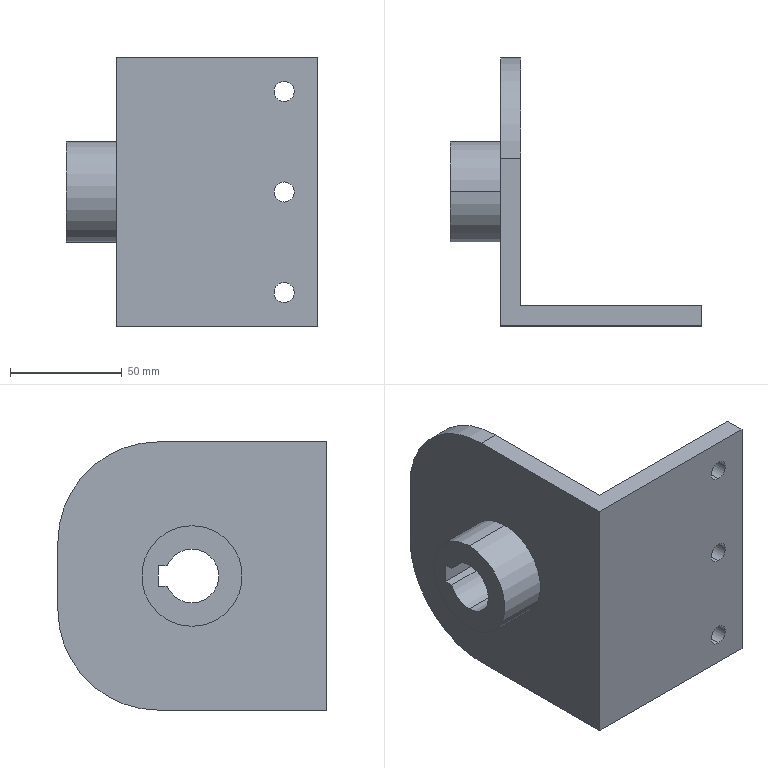Part | SolidWorks | features ICE 2, BaseBody 1 | 1 solid | 25 faces | box 112.5 x 120 x 120 mm | volume 228143 mm3 | cylinder 13 | plane 12 | commonest cylinder face diameters 9 x6 24 x3 45 x2 90 x2
STEP:
#1=CARTESIAN_POINT('',(75.,0.,40.5));
#2=VERTEX_POINT('',#1);
#3=CARTESIAN_POINT('',(75.,0.,49.5));
#4=VERTEX_POINT('',#3);
#5=CARTESIAN_POINT('',(75.,0.,45.));
#6=DIRECTION('',(0.,1.,0.));
#7=DIRECTION('',(0.,0.,-1.));
#8=AXIS2_PLACEMENT_3D('',#5,#6,#7);
#9=CIRCLE('',#8,4.5);
#10=EDGE_CURVE('',#2,#4,#9,.T.);
#11=ORIENTED_EDGE('',*,*,#10,.F.);
#12=CARTESIAN_POINT('',(75.,9.,40.5));
#13=VERTEX_POINT('',#12);
#14=CARTESIAN_POINT('',(75.,-14.849,40.5));
#15=DIRECTION('',(0.,1.,0.));
#16=VECTOR('',#15,1000.);
#17=LINE('',#14,#16);
#18=EDGE_CURVE('',#2,#13,#17,.T.);
#19=ORIENTED_EDGE('',*,*,#18,.T.);
#20=CARTESIAN_POINT('',(75.,9.,49.5));
#21=VERTEX_POINT('',#20);
#22=CARTESIAN_POINT('',(75.,9.,45.));
#23=DIRECTION('',(0.,1.,0.));
#24=DIRECTION('',(0.,0.,1.));
#25=AXIS2_PLACEMENT_3D('',#22,#23,#24);
#26=CIRCLE('',#25,4.5);
#27=EDGE_CURVE('',#13,#21,#26,.T.);
#28=ORIENTED_EDGE('',*,*,#27,.T.);
#29=CARTESIAN_POINT('',(75.,-14.849,49.5));
#30=DIRECTION('',(0.,1.,0.));
#31=VECTOR('',#30,1000.);
#32=LINE('',#29,#31);
#33=EDGE_CURVE('',#4,#21,#32,.T.);
#34=ORIENTED_EDGE('',*,*,#33,.F.);
#35=EDGE_LOOP('',(#11,#19,#28,#34));
#36=FACE_OUTER_BOUND('',#35,.T.);
#37=CARTESIAN_POINT('',(75.,-14.849,45.));
#38=DIRECTION('',(0.,1.,0.));
#39=DIRECTION('',(0.,0.,1.));
#40=AXIS2_PLACEMENT_3D('',#37,#38,#39);
#41=CYLINDRICAL_SURFACE('',#40,4.5);
#42=ADVANCED_FACE('',(#36),#41,.F.);
#43=CARTESIAN_POINT('',(75.,0.,-4.5));
#44=VERTEX_POINT('',#43);
#45=CARTESIAN_POINT('',(75.,0.,4.5));
#46=VERTEX_POINT('',#45);
#47=CARTESIAN_POINT('',(75.,0.,0.));
#48=DIRECTION('',(0.,1.,0.));
#49=DIRECTION('',(0.,0.,-1.));
#50=AXIS2_PLACEMENT_3D('',#47,#48,#49);
#51=CIRCLE('',#50,4.5);
#52=EDGE_CURVE('',#44,#46,#51,.T.);
#53=ORIENTED_EDGE('',*,*,#52,.F.);
#54=CARTESIAN_POINT('',(75.,9.,-4.5));
#55=VERTEX_POINT('',#54);
#56=CARTESIAN_POINT('',(75.,-14.849,-4.5));
#57=DIRECTION('',(0.,1.,0.));
#58=VECTOR('',#57,1000.);
#59=LINE('',#56,#58);
#60=EDGE_CURVE('',#44,#55,#59,.T.);
#61=ORIENTED_EDGE('',*,*,#60,.T.);
#62=CARTESIAN_POINT('',(75.,9.,4.5));
#63=VERTEX_POINT('',#62);
#64=CARTESIAN_POINT('',(75.,9.,0.));
#65=DIRECTION('',(0.,1.,0.));
#66=DIRECTION('',(0.,0.,1.));
#67=AXIS2_PLACEMENT_3D('',#64,#65,#66);
#68=CIRCLE('',#67,4.5);
#69=EDGE_CURVE('',#55,#63,#68,.T.);
#70=ORIENTED_EDGE('',*,*,#69,.T.);
#71=CARTESIAN_POINT('',(75.,-14.849,4.5));
#72=DIRECTION('',(0.,1.,0.));
#73=VECTOR('',#72,1000.);
#74=LINE('',#71,#73);
#75=EDGE_CURVE('',#46,#63,#74,.T.);
#76=ORIENTED_EDGE('',*,*,#75,.F.);
#77=EDGE_LOOP('',(#53,#61,#70,#76));
#78=FACE_OUTER_BOUND('',#77,.T.);
#79=CARTESIAN_POINT('',(75.,-14.849,0.));
#80=DIRECTION('',(0.,1.,0.));
#81=DIRECTION('',(0.,0.,1.));
#82=AXIS2_PLACEMENT_3D('',#79,#80,#81);
#83=CYLINDRICAL_SURFACE('',#82,4.5);
#84=ADVANCED_FACE('',(#78),#83,.F.);
#85=CARTESIAN_POINT('',(75.,0.,-49.5));
#86=VERTEX_POINT('',#85);
#87=CARTESIAN_POINT('',(75.,0.,-40.5));
#88=VERTEX_POINT('',#87);
#89=CARTESIAN_POINT('',(75.,0.,-45.));
#90=DIRECTION('',(0.,1.,0.));
#91=DIRECTION('',(0.,0.,-1.));
#92=AXIS2_PLACEMENT_3D('',#89,#90,#91);
#93=CIRCLE('',#92,4.5);
#94=EDGE_CURVE('',#86,#88,#93,.T.);
#95=ORIENTED_EDGE('',*,*,#94,.F.);
#96=CARTESIAN_POINT('',(75.,9.,-49.5));
#97=VERTEX_POINT('',#96);
#98=CARTESIAN_POINT('',(75.,-14.849,-49.5));
#99=DIRECTION('',(0.,1.,0.));
#100=VECTOR('',#99,1000.);
#101=LINE('',#98,#100);
#102=EDGE_CURVE('',#86,#97,#101,.T.);
#103=ORIENTED_EDGE('',*,*,#102,.T.);
#104=CARTESIAN_POINT('',(75.,9.,-40.5));
#105=VERTEX_POINT('',#104);
#106=CARTESIAN_POINT('',(75.,9.,-45.));
#107=DIRECTION('',(0.,1.,0.));
#108=DIRECTION('',(0.,0.,1.));
#109=AXIS2_PLACEMENT_3D('',#106,#107,#108);
#110=CIRCLE('',#109,4.5);
#111=EDGE_CURVE('',#97,#105,#110,.T.);
#112=ORIENTED_EDGE('',*,*,#111,.T.);
#113=CARTESIAN_POINT('',(75.,-14.849,-40.5));
#114=DIRECTION('',(0.,1.,0.));
#115=VECTOR('',#114,1000.);
#116=LINE('',#113,#115);
#117=EDGE_CURVE('',#88,#105,#116,.T.);
#118=ORIENTED_EDGE('',*,*,#117,.F.);
#119=EDGE_LOOP('',(#95,#103,#112,#118));
#120=FACE_OUTER_BOUND('',#119,.T.);
#121=CARTESIAN_POINT('',(75.,-14.849,-45.));
#122=DIRECTION('',(0.,1.,0.));
#123=DIRECTION('',(0.,0.,1.));
#124=AXIS2_PLACEMENT_3D('',#121,#122,#123);
#125=CYLINDRICAL_SURFACE('',#124,4.5);
#126=ADVANCED_FACE('',(#120),#125,.F.);
#127=CARTESIAN_POINT('',(0.,60.,-22.5));
#128=VERTEX_POINT('',#127);
#129=CARTESIAN_POINT('',(0.,60.,22.5));
#130=VERTEX_POINT('',#129);
#131=CARTESIAN_POINT('',(0.,60.,0.));
#132=DIRECTION('',(1.,0.,0.));
#133=DIRECTION('',(0.,0.,1.));
#134=AXIS2_PLACEMENT_3D('',#131,#132,#133);
#135=CIRCLE('',#134,22.5);
#136=EDGE_CURVE('',#128,#130,#135,.T.);
#137=ORIENTED_EDGE('',*,*,#136,.F.);
#138=CARTESIAN_POINT('',(-22.5,60.,-22.5));
#139=VERTEX_POINT('',#138);
#140=CARTESIAN_POINT('',(72.125,60.,-22.5));
#141=DIRECTION('',(-1.,0.,0.));
#142=VECTOR('',#141,1000.);
#143=LINE('',#140,#142);
#144=EDGE_CURVE('',#128,#139,#143,.T.);
#145=ORIENTED_EDGE('',*,*,#144,.T.);
#146=CARTESIAN_POINT('',(-22.5,60.,22.5));
#147=VERTEX_POINT('',#146);
#148=CARTESIAN_POINT('',(-22.5,60.,0.));
#149=DIRECTION('',(-1.,0.,0.));
#150=DIRECTION('',(0.,0.,1.));
#151=AXIS2_PLACEMENT_3D('',#148,#149,#150);
#152=CIRCLE('',#151,22.5);
#153=EDGE_CURVE('',#147,#139,#152,.T.);
#154=ORIENTED_EDGE('',*,*,#153,.F.);
#155=CARTESIAN_POINT('',(72.125,60.,22.5));
#156=DIRECTION('',(-1.,0.,0.));
#157=VECTOR('',#156,1000.);
#158=LINE('',#155,#157);
#159=EDGE_CURVE('',#130,#147,#158,.T.);
#160=ORIENTED_EDGE('',*,*,#159,.F.);
#161=EDGE_LOOP('',(#137,#145,#154,#160));
#162=FACE_OUTER_BOUND('',#161,.T.);
#163=CARTESIAN_POINT('',(72.125,60.,0.));
#164=DIRECTION('',(-1.,0.,0.));
#165=DIRECTION('',(0.,0.,1.));
#166=AXIS2_PLACEMENT_3D('',#163,#164,#165);
#167=CYLINDRICAL_SURFACE('',#166,22.5);
#168=ADVANCED_FACE('',(#162),#167,.T.);
#169=CARTESIAN_POINT('',(9.,60.,12.));
#170=VERTEX_POINT('',#169);
#171=CARTESIAN_POINT('',(9.,60.,-12.));
#172=VERTEX_POINT('',#171);
#173=CARTESIAN_POINT('',(9.,60.,0.));
#174=DIRECTION('',(1.,0.,0.));
#175=DIRECTION('',(0.,0.,1.));
#176=AXIS2_PLACEMENT_3D('',#173,#174,#175);
#177=CIRCLE('',#176,12.);
#178=EDGE_CURVE('',#170,#172,#177,.T.);
#179=ORIENTED_EDGE('',*,*,#178,.T.);
#180=CARTESIAN_POINT('',(-22.5,60.,-12.));
#181=VERTEX_POINT('',#180);
#182=CARTESIAN_POINT('',(9.,60.,-12.));
#183=DIRECTION('',(-1.,0.,0.));
#184=VECTOR('',#183,1000.);
#185=LINE('',#182,#184);
#186=EDGE_CURVE('',#172,#181,#185,.T.);
#187=ORIENTED_EDGE('',*,*,#186,.T.);
#188=CARTESIAN_POINT('',(-22.5,60.,12.));
#189=VERTEX_POINT('',#188);
#190=CARTESIAN_POINT('',(-22.5,60.,0.));
#191=DIRECTION('',(-1.,0.,0.));
#192=DIRECTION('',(0.,0.,1.));
#193=AXIS2_PLACEMENT_3D('',#190,#191,#192);
#194=CIRCLE('',#193,12.);
#195=EDGE_CURVE('',#181,#189,#194,.T.);
#196=ORIENTED_EDGE('',*,*,#195,.T.);
#197=CARTESIAN_POINT('',(9.,60.,12.));
#198=DIRECTION('',(-1.,0.,0.));
#199=VECTOR('',#198,1000.);
#200=LINE('',#197,#199);
#201=EDGE_CURVE('',#170,#189,#200,.T.);
#202=ORIENTED_EDGE('',*,*,#201,.F.);
#203=EDGE_LOOP('',(#179,#187,#196,#202));
#204=FACE_OUTER_BOUND('',#203,.T.);
#205=CARTESIAN_POINT('',(9.,60.,0.));
#206=DIRECTION('',(-1.,0.,0.));
#207=DIRECTION('',(0.,0.,1.));
#208=AXIS2_PLACEMENT_3D('',#205,#206,#207);
#209=CYLINDRICAL_SURFACE('',#208,12.);
#210=ADVANCED_FACE('',(#204),#209,.F.);
#211=CARTESIAN_POINT('',(9.,71.124,4.5));
#212=VERTEX_POINT('',#211);
#213=CARTESIAN_POINT('',(9.,60.,0.));
#214=DIRECTION('',(1.,0.,0.));
#215=DIRECTION('',(0.,0.,1.));
#216=AXIS2_PLACEMENT_3D('',#213,#214,#215);
#217=CIRCLE('',#216,12.);
#218=EDGE_CURVE('',#212,#170,#217,.T.);
#219=ORIENTED_EDGE('',*,*,#218,.T.);
#220=ORIENTED_EDGE('',*,*,#201,.T.);
#221=CARTESIAN_POINT('',(-22.5,71.124,4.5));
#222=VERTEX_POINT('',#221);
#223=CARTESIAN_POINT('',(-22.5,60.,0.));
#224=DIRECTION('',(-1.,0.,0.));
#225=DIRECTION('',(0.,0.,1.));
#226=AXIS2_PLACEMENT_3D('',#223,#224,#225);
#227=CIRCLE('',#226,12.);
#228=EDGE_CURVE('',#189,#222,#227,.T.);
#229=ORIENTED_EDGE('',*,*,#228,.T.);
#230=CARTESIAN_POINT('',(-6.75,71.124,4.5));
#231=DIRECTION('',(1.,0.,0.));
#232=VECTOR('',#231,1000.);
#233=LINE('',#230,#232);
#234=EDGE_CURVE('',#222,#212,#233,.T.);
#235=ORIENTED_EDGE('',*,*,#234,.T.);
#236=EDGE_LOOP('',(#219,#220,#229,#235));
#237=FACE_OUTER_BOUND('',#236,.T.);
#238=CARTESIAN_POINT('',(9.,60.,0.));
#239=DIRECTION('',(-1.,0.,0.));
#240=DIRECTION('',(0.,0.,1.));
#241=AXIS2_PLACEMENT_3D('',#238,#239,#240);
#242=CYLINDRICAL_SURFACE('',#241,12.);
#243=ADVANCED_FACE('',(#237),#242,.F.);
#244=CARTESIAN_POINT('',(-22.5,75.,-4.5));
#245=VERTEX_POINT('',#244);
#246=CARTESIAN_POINT('',(-22.5,75.,4.5));
#247=VERTEX_POINT('',#246);
#248=CARTESIAN_POINT('',(-22.5,75.,0.));
#249=DIRECTION('',(0.,0.,1.));
#250=VECTOR('',#249,1000.);
#251=LINE('',#248,#250);
#252=EDGE_CURVE('',#245,#247,#251,.T.);
#253=ORIENTED_EDGE('',*,*,#252,.T.);
#254=CARTESIAN_POINT('',(-22.5,60.,4.5));
#255=DIRECTION('',(0.,-1.,0.));
#256=VECTOR('',#255,1000.);
#257=LINE('',#254,#256);
#258=EDGE_CURVE('',#247,#222,#257,.T.);
#259=ORIENTED_EDGE('',*,*,#258,.T.);
#260=ORIENTED_EDGE('',*,*,#228,.F.);
#261=ORIENTED_EDGE('',*,*,#195,.F.);
#262=CARTESIAN_POINT('',(-22.5,71.124,-4.5));
#263=VERTEX_POINT('',#262);
#264=CARTESIAN_POINT('',(-22.5,60.,0.));
#265=DIRECTION('',(-1.,0.,0.));
#266=DIRECTION('',(0.,0.,1.));
#267=AXIS2_PLACEMENT_3D('',#264,#265,#266);
#268=CIRCLE('',#267,12.);
#269=EDGE_CURVE('',#263,#181,#268,.T.);
#270=ORIENTED_EDGE('',*,*,#269,.F.);
#271=CARTESIAN_POINT('',(-22.5,60.,-4.5));
#272=DIRECTION('',(0.,1.,0.));
#273=VECTOR('',#272,1000.);
#274=LINE('',#271,#273);
#275=EDGE_CURVE('',#263,#245,#274,.T.);
#276=ORIENTED_EDGE('',*,*,#275,.T.);
#277=EDGE_LOOP('',(#253,#259,#260,#261,#270,#276));
#278=FACE_BOUND('',#277,.T.);
#279=ORIENTED_EDGE('',*,*,#153,.T.);
#280=CARTESIAN_POINT('',(-22.5,60.,0.));
#281=DIRECTION('',(-1.,0.,0.));
#282=DIRECTION('',(0.,0.,1.));
#283=AXIS2_PLACEMENT_3D('',#280,#281,#282);
#284=CIRCLE('',#283,22.5);
#285=EDGE_CURVE('',#139,#147,#284,.T.);
#286=ORIENTED_EDGE('',*,*,#285,.T.);
#287=EDGE_LOOP('',(#279,#286));
#288=FACE_OUTER_BOUND('',#287,.T.);
#289=CARTESIAN_POINT('',(-22.5,34.194,-25.806));
#290=DIRECTION('',(-1.,0.,0.));
#291=DIRECTION('',(0.,0.,1.));
#292=AXIS2_PLACEMENT_3D('',#289,#290,#291);
#293=PLANE('',#292);
#294=ADVANCED_FACE('',(#278,#288),#293,.T.);
#295=ORIENTED_EDGE('',*,*,#186,.F.);
#296=CARTESIAN_POINT('',(9.,71.124,-4.5));
#297=VERTEX_POINT('',#296);
#298=CARTESIAN_POINT('',(9.,60.,0.));
#299=DIRECTION('',(1.,0.,0.));
#300=DIRECTION('',(0.,0.,1.));
#301=AXIS2_PLACEMENT_3D('',#298,#299,#300);
#302=CIRCLE('',#301,12.);
#303=EDGE_CURVE('',#172,#297,#302,.T.);
#304=ORIENTED_EDGE('',*,*,#303,.T.);
#305=CARTESIAN_POINT('',(-6.75,71.124,-4.5));
#306=DIRECTION('',(-1.,0.,0.));
#307=VECTOR('',#306,1000.);
#308=LINE('',#305,#307);
#309=EDGE_CURVE('',#297,#263,#308,.T.);
#310=ORIENTED_EDGE('',*,*,#309,.T.);
#311=ORIENTED_EDGE('',*,*,#269,.T.);
#312=EDGE_LOOP('',(#295,#304,#310,#311));
#313=FACE_OUTER_BOUND('',#312,.T.);
#314=CARTESIAN_POINT('',(9.,60.,0.));
#315=DIRECTION('',(-1.,0.,0.));
#316=DIRECTION('',(0.,0.,1.));
#317=AXIS2_PLACEMENT_3D('',#314,#315,#316);
#318=CYLINDRICAL_SURFACE('',#317,12.);
#319=ADVANCED_FACE('',(#313),#318,.F.);
#320=CARTESIAN_POINT('',(9.,75.,-4.5));
#321=VERTEX_POINT('',#320);
#322=CARTESIAN_POINT('',(9.,75.,4.5));
#323=VERTEX_POINT('',#322);
#324=CARTESIAN_POINT('',(9.,75.,0.));
#325=DIRECTION('',(0.,0.,1.));
#326=VECTOR('',#325,1000.);
#327=LINE('',#324,#326);
#328=EDGE_CURVE('',#321,#323,#327,.T.);
#329=ORIENTED_EDGE('',*,*,#328,.F.);
#330=CARTESIAN_POINT('',(9.,64.5,-4.5));
#331=DIRECTION('',(0.,1.,0.));
#332=VECTOR('',#331,1000.);
#333=LINE('',#330,#332);
#334=EDGE_CURVE('',#297,#321,#333,.T.);
#335=ORIENTED_EDGE('',*,*,#334,.F.);
#336=ORIENTED_EDGE('',*,*,#303,.F.);
#337=ORIENTED_EDGE('',*,*,#178,.F.);
#338=ORIENTED_EDGE('',*,*,#218,.F.);
#339=CARTESIAN_POINT('',(9.,64.5,4.5));
#340=DIRECTION('',(0.,-1.,0.));
#341=VECTOR('',#340,1000.);
#342=LINE('',#339,#341);
#343=EDGE_CURVE('',#323,#212,#342,.T.);
#344=ORIENTED_EDGE('',*,*,#343,.F.);
#345=EDGE_LOOP('',(#329,#335,#336,#337,#338,#344));
#346=FACE_BOUND('',#345,.T.);
#347=CARTESIAN_POINT('',(9.,75.,60.));
#348=VERTEX_POINT('',#347);
#349=CARTESIAN_POINT('',(9.,120.,15.));
#350=VERTEX_POINT('',#349);
#351=CARTESIAN_POINT('',(9.,75.,15.));
#352=DIRECTION('',(-1.,0.,0.));
#353=DIRECTION('',(0.,0.,1.));
#354=AXIS2_PLACEMENT_3D('',#351,#352,#353);
#355=CIRCLE('',#354,45.);
#356=EDGE_CURVE('',#348,#350,#355,.T.);
#357=ORIENTED_EDGE('',*,*,#356,.F.);
#358=CARTESIAN_POINT('',(9.,9.,60.));
#359=VERTEX_POINT('',#358);
#360=CARTESIAN_POINT('',(9.,64.5,60.));
#361=DIRECTION('',(0.,1.,0.));
#362=VECTOR('',#361,1000.);
#363=LINE('',#360,#362);
#364=EDGE_CURVE('',#359,#348,#363,.T.);
#365=ORIENTED_EDGE('',*,*,#364,.F.);
#366=CARTESIAN_POINT('',(9.,9.,-60.));
#367=VERTEX_POINT('',#366);
#368=CARTESIAN_POINT('',(9.,9.,0.));
#369=DIRECTION('',(0.,0.,1.));
#370=VECTOR('',#369,1000.);
#371=LINE('',#368,#370);
#372=EDGE_CURVE('',#367,#359,#371,.T.);
#373=ORIENTED_EDGE('',*,*,#372,.F.);
#374=CARTESIAN_POINT('',(9.,75.,-60.));
#375=VERTEX_POINT('',#374);
#376=CARTESIAN_POINT('',(9.,64.5,-60.));
#377=DIRECTION('',(0.,-1.,0.));
#378=VECTOR('',#377,1000.);
#379=LINE('',#376,#378);
#380=EDGE_CURVE('',#375,#367,#379,.T.);
#381=ORIENTED_EDGE('',*,*,#380,.F.);
#382=CARTESIAN_POINT('',(9.,120.,-15.));
#383=VERTEX_POINT('',#382);
#384=CARTESIAN_POINT('',(9.,75.,-15.));
#385=DIRECTION('',(-1.,0.,0.));
#386=DIRECTION('',(0.,0.,-1.));
#387=AXIS2_PLACEMENT_3D('',#384,#385,#386);
#388=CIRCLE('',#387,45.);
#389=EDGE_CURVE('',#383,#375,#388,.T.);
#390=ORIENTED_EDGE('',*,*,#389,.F.);
#391=CARTESIAN_POINT('',(9.,120.,0.));
#392=DIRECTION('',(0.,0.,-1.));
#393=VECTOR('',#392,1000.);
#394=LINE('',#391,#393);
#395=EDGE_CURVE('',#350,#383,#394,.T.);
#396=ORIENTED_EDGE('',*,*,#395,.F.);
#397=EDGE_LOOP('',(#357,#365,#373,#381,#390,#396));
#398=FACE_OUTER_BOUND('',#397,.T.);
#399=CARTESIAN_POINT('',(9.,9.,-60.));
#400=DIRECTION('',(-1.,0.,0.));
#401=DIRECTION('',(0.,0.,1.));
#402=AXIS2_PLACEMENT_3D('',#399,#400,#401);
#403=PLANE('',#402);
#404=ADVANCED_FACE('',(#346,#398),#403,.F.);
#405=ORIENTED_EDGE('',*,*,#234,.F.);
#406=ORIENTED_EDGE('',*,*,#258,.F.);
#407=CARTESIAN_POINT('',(-6.75,75.,4.5));
#408=DIRECTION('',(-1.,0.,0.));
#409=VECTOR('',#408,1000.);
#410=LINE('',#407,#409);
#411=EDGE_CURVE('',#323,#247,#410,.T.);
#412=ORIENTED_EDGE('',*,*,#411,.F.);
#413=ORIENTED_EDGE('',*,*,#343,.T.);
#414=EDGE_LOOP('',(#405,#406,#412,#413));
#415=FACE_OUTER_BOUND('',#414,.T.);
#416=CARTESIAN_POINT('',(-22.5,71.124,4.5));
#417=DIRECTION('',(0.,0.,1.));
#418=DIRECTION('',(1.,0.,0.));
#419=AXIS2_PLACEMENT_3D('',#416,#417,#418);
#420=PLANE('',#419);
#421=ADVANCED_FACE('',(#415),#420,.F.);
#422=CARTESIAN_POINT('',(-6.75,75.,-4.5));
#423=DIRECTION('',(-1.,0.,0.));
#424=VECTOR('',#423,1000.);
#425=LINE('',#422,#424);
#426=EDGE_CURVE('',#321,#245,#425,.T.);
#427=ORIENTED_EDGE('',*,*,#426,.F.);
#428=ORIENTED_EDGE('',*,*,#328,.T.);
#429=ORIENTED_EDGE('',*,*,#411,.T.);
#430=ORIENTED_EDGE('',*,*,#252,.F.);
#431=EDGE_LOOP('',(#427,#428,#429,#430));
#432=FACE_OUTER_BOUND('',#431,.T.);
#433=CARTESIAN_POINT('',(-22.5,75.,-4.5));
#434=DIRECTION('',(0.,1.,0.));
#435=DIRECTION('',(0.,0.,1.));
#436=AXIS2_PLACEMENT_3D('',#433,#434,#435);
#437=PLANE('',#436);
#438=ADVANCED_FACE('',(#432),#437,.F.);
#439=ORIENTED_EDGE('',*,*,#309,.F.);
#440=ORIENTED_EDGE('',*,*,#334,.T.);
#441=ORIENTED_EDGE('',*,*,#426,.T.);
#442=ORIENTED_EDGE('',*,*,#275,.F.);
#443=EDGE_LOOP('',(#439,#440,#441,#442));
#444=FACE_OUTER_BOUND('',#443,.T.);
#445=CARTESIAN_POINT('',(9.,71.124,-4.5));
#446=DIRECTION('',(0.,0.,-1.));
#447=DIRECTION('',(-1.,0.,0.));
#448=AXIS2_PLACEMENT_3D('',#445,#446,#447);
#449=PLANE('',#448);
#450=ADVANCED_FACE('',(#444),#449,.F.);
#451=CARTESIAN_POINT('',(0.,120.,-15.));
#452=VERTEX_POINT('',#451);
#453=CARTESIAN_POINT('',(0.,120.,15.));
#454=VERTEX_POINT('',#453);
#455=CARTESIAN_POINT('',(0.,120.,0.));
#456=DIRECTION('',(0.,0.,1.));
#457=VECTOR('',#456,1000.);
#458=LINE('',#455,#457);
#459=EDGE_CURVE('',#452,#454,#458,.T.);
#460=ORIENTED_EDGE('',*,*,#459,.T.);
#461=CARTESIAN_POINT('',(4.5,120.,15.));
#462=DIRECTION('',(1.,0.,0.));
#463=VECTOR('',#462,1000.);
#464=LINE('',#461,#463);
#465=EDGE_CURVE('',#454,#350,#464,.T.);
#466=ORIENTED_EDGE('',*,*,#465,.T.);
#467=ORIENTED_EDGE('',*,*,#395,.T.);
#468=CARTESIAN_POINT('',(4.5,120.,-15.));
#469=DIRECTION('',(-1.,0.,0.));
#470=VECTOR('',#469,1000.);
#471=LINE('',#468,#470);
#472=EDGE_CURVE('',#383,#452,#471,.T.);
#473=ORIENTED_EDGE('',*,*,#472,.T.);
#474=EDGE_LOOP('',(#460,#466,#467,#473));
#475=FACE_OUTER_BOUND('',#474,.T.);
#476=CARTESIAN_POINT('',(0.,120.,-15.));
#477=DIRECTION('',(0.,1.,0.));
#478=DIRECTION('',(0.,0.,1.));
#479=AXIS2_PLACEMENT_3D('',#476,#477,#478);
#480=PLANE('',#479);
#481=ADVANCED_FACE('',(#475),#480,.T.);
#482=CARTESIAN_POINT('',(0.,75.,60.));
#483=VERTEX_POINT('',#482);
#484=CARTESIAN_POINT('',(0.,75.,15.));
#485=DIRECTION('',(-1.,0.,0.));
#486=DIRECTION('',(0.,0.,1.));
#487=AXIS2_PLACEMENT_3D('',#484,#485,#486);
#488=CIRCLE('',#487,45.);
#489=EDGE_CURVE('',#483,#454,#488,.T.);
#490=ORIENTED_EDGE('',*,*,#489,.F.);
#491=CARTESIAN_POINT('',(4.5,75.,60.));
#492=DIRECTION('',(-1.,0.,0.));
#493=VECTOR('',#492,1000.);
#494=LINE('',#491,#493);
#495=EDGE_CURVE('',#348,#483,#494,.T.);
#496=ORIENTED_EDGE('',*,*,#495,.F.);
#497=ORIENTED_EDGE('',*,*,#356,.T.);
#498=ORIENTED_EDGE('',*,*,#465,.F.);
#499=EDGE_LOOP('',(#490,#496,#497,#498));
#500=FACE_OUTER_BOUND('',#499,.T.);
#501=CARTESIAN_POINT('',(9.,75.,15.));
#502=DIRECTION('',(-1.,0.,0.));
#503=DIRECTION('',(0.,0.,1.));
#504=AXIS2_PLACEMENT_3D('',#501,#502,#503);
#505=CYLINDRICAL_SURFACE('',#504,45.);
#506=ADVANCED_FACE('',(#500),#505,.T.);
#507=CARTESIAN_POINT('',(90.,0.,60.));
#508=VERTEX_POINT('',#507);
#509=CARTESIAN_POINT('',(0.,0.,60.));
#510=VERTEX_POINT('',#509);
#511=CARTESIAN_POINT('',(45.,0.,60.));
#512=DIRECTION('',(-1.,0.,0.));
#513=VECTOR('',#512,1000.);
#514=LINE('',#511,#513);
#515=EDGE_CURVE('',#508,#510,#514,.T.);
#516=ORIENTED_EDGE('',*,*,#515,.F.);
#517=CARTESIAN_POINT('',(90.,9.,60.));
#518=VERTEX_POINT('',#517);
#519=CARTESIAN_POINT('',(90.,37.5,60.));
#520=DIRECTION('',(0.,-1.,0.));
#521=VECTOR('',#520,1000.);
#522=LINE('',#519,#521);
#523=EDGE_CURVE('',#518,#508,#522,.T.);
#524=ORIENTED_EDGE('',*,*,#523,.F.);
#525=CARTESIAN_POINT('',(45.,9.,60.));
#526=DIRECTION('',(1.,0.,0.));
#527=VECTOR('',#526,1000.);
#528=LINE('',#525,#527);
#529=EDGE_CURVE('',#359,#518,#528,.T.);
#530=ORIENTED_EDGE('',*,*,#529,.F.);
#531=ORIENTED_EDGE('',*,*,#364,.T.);
#532=ORIENTED_EDGE('',*,*,#495,.T.);
#533=CARTESIAN_POINT('',(0.,37.5,60.));
#534=DIRECTION('',(0.,1.,0.));
#535=VECTOR('',#534,1000.);
#536=LINE('',#533,#535);
#537=EDGE_CURVE('',#510,#483,#536,.T.);
#538=ORIENTED_EDGE('',*,*,#537,.F.);
#539=EDGE_LOOP('',(#516,#524,#530,#531,#532,#538));
#540=FACE_OUTER_BOUND('',#539,.T.);
#541=CARTESIAN_POINT('',(90.,0.,60.));
#542=DIRECTION('',(0.,0.,-1.));
#543=DIRECTION('',(-1.,0.,0.));
#544=AXIS2_PLACEMENT_3D('',#541,#542,#543);
#545=PLANE('',#544);
#546=ADVANCED_FACE('',(#540),#545,.F.);
#547=CARTESIAN_POINT('',(90.,9.,-60.));
#548=VERTEX_POINT('',#547);
#549=CARTESIAN_POINT('',(90.,9.,0.));
#550=DIRECTION('',(0.,0.,1.));
#551=VECTOR('',#550,1000.);
#552=LINE('',#549,#551);
#553=EDGE_CURVE('',#548,#518,#552,.T.);
#554=ORIENTED_EDGE('',*,*,#553,.F.);
#555=CARTESIAN_POINT('',(49.5,9.,-60.));
#556=DIRECTION('',(1.,0.,0.));
#557=VECTOR('',#556,1000.);
#558=LINE('',#555,#557);
#559=EDGE_CURVE('',#367,#548,#558,.T.);
#560=ORIENTED_EDGE('',*,*,#559,.F.);
#561=ORIENTED_EDGE('',*,*,#372,.T.);
#562=ORIENTED_EDGE('',*,*,#529,.T.);
#563=EDGE_LOOP('',(#554,#560,#561,#562));
#564=FACE_OUTER_BOUND('',#563,.T.);
#565=CARTESIAN_POINT('',(75.,9.,-45.));
#566=DIRECTION('',(0.,1.,0.));
#567=DIRECTION('',(0.,0.,1.));
#568=AXIS2_PLACEMENT_3D('',#565,#566,#567);
#569=CIRCLE('',#568,4.5);
#570=EDGE_CURVE('',#105,#97,#569,.T.);
#571=ORIENTED_EDGE('',*,*,#570,.F.);
#572=ORIENTED_EDGE('',*,*,#111,.F.);
#573=EDGE_LOOP('',(#571,#572));
#574=FACE_BOUND('',#573,.T.);
#575=CARTESIAN_POINT('',(75.,9.,0.));
#576=DIRECTION('',(0.,1.,0.));
#577=DIRECTION('',(0.,0.,1.));
#578=AXIS2_PLACEMENT_3D('',#575,#576,#577);
#579=CIRCLE('',#578,4.5);
#580=EDGE_CURVE('',#63,#55,#579,.T.);
#581=ORIENTED_EDGE('',*,*,#580,.F.);
#582=ORIENTED_EDGE('',*,*,#69,.F.);
#583=EDGE_LOOP('',(#581,#582));
#584=FACE_BOUND('',#583,.T.);
#585=CARTESIAN_POINT('',(75.,9.,45.));
#586=DIRECTION('',(0.,1.,0.));
#587=DIRECTION('',(0.,0.,1.));
#588=AXIS2_PLACEMENT_3D('',#585,#586,#587);
#589=CIRCLE('',#588,4.5);
#590=EDGE_CURVE('',#21,#13,#589,.T.);
#591=ORIENTED_EDGE('',*,*,#590,.F.);
#592=ORIENTED_EDGE('',*,*,#27,.F.);
#593=EDGE_LOOP('',(#591,#592));
#594=FACE_BOUND('',#593,.T.);
#595=CARTESIAN_POINT('',(9.,9.,60.));
#596=DIRECTION('',(0.,-1.,0.));
#597=DIRECTION('',(0.,0.,-1.));
#598=AXIS2_PLACEMENT_3D('',#595,#596,#597);
#599=PLANE('',#598);
#600=ADVANCED_FACE('',(#564,#574,#584,#594),#599,.F.);
#601=CARTESIAN_POINT('',(0.,0.,-60.));
#602=VERTEX_POINT('',#601);
#603=CARTESIAN_POINT('',(0.,75.,-60.));
#604=VERTEX_POINT('',#603);
#605=CARTESIAN_POINT('',(0.,37.5,-60.));
#606=DIRECTION('',(0.,1.,0.));
#607=VECTOR('',#606,1000.);
#608=LINE('',#605,#607);
#609=EDGE_CURVE('',#602,#604,#608,.T.);
#610=ORIENTED_EDGE('',*,*,#609,.T.);
#611=CARTESIAN_POINT('',(45.,75.,-60.));
#612=DIRECTION('',(1.,0.,0.));
#613=VECTOR('',#612,1000.);
#614=LINE('',#611,#613);
#615=EDGE_CURVE('',#604,#375,#614,.T.);
#616=ORIENTED_EDGE('',*,*,#615,.T.);
#617=ORIENTED_EDGE('',*,*,#380,.T.);
#618=ORIENTED_EDGE('',*,*,#559,.T.);
#619=CARTESIAN_POINT('',(90.,0.,-60.));
#620=VERTEX_POINT('',#619);
#621=CARTESIAN_POINT('',(90.,37.5,-60.));
#622=DIRECTION('',(0.,-1.,0.));
#623=VECTOR('',#622,1000.);
#624=LINE('',#621,#623);
#625=EDGE_CURVE('',#548,#620,#624,.T.);
#626=ORIENTED_EDGE('',*,*,#625,.T.);
#627=CARTESIAN_POINT('',(45.,0.,-60.));
#628=DIRECTION('',(-1.,0.,0.));
#629=VECTOR('',#628,1000.);
#630=LINE('',#627,#629);
#631=EDGE_CURVE('',#620,#602,#630,.T.);
#632=ORIENTED_EDGE('',*,*,#631,.T.);
#633=EDGE_LOOP('',(#610,#616,#617,#618,#626,#632));
#634=FACE_OUTER_BOUND('',#633,.T.);
#635=CARTESIAN_POINT('',(90.,0.,-60.));
#636=DIRECTION('',(0.,0.,-1.));
#637=DIRECTION('',(-1.,0.,0.));
#638=AXIS2_PLACEMENT_3D('',#635,#636,#637);
#639=PLANE('',#638);
#640=ADVANCED_FACE('',(#634),#639,.T.);
#641=CARTESIAN_POINT('',(0.,75.,-15.));
#642=DIRECTION('',(-1.,0.,0.));
#643=DIRECTION('',(0.,0.,-1.));
#644=AXIS2_PLACEMENT_3D('',#641,#642,#643);
#645=CIRCLE('',#644,45.);
#646=EDGE_CURVE('',#452,#604,#645,.T.);
#647=ORIENTED_EDGE('',*,*,#646,.F.);
#648=ORIENTED_EDGE('',*,*,#472,.F.);
#649=ORIENTED_EDGE('',*,*,#389,.T.);
#650=ORIENTED_EDGE('',*,*,#615,.F.);
#651=EDGE_LOOP('',(#647,#648,#649,#650));
#652=FACE_OUTER_BOUND('',#651,.T.);
#653=CARTESIAN_POINT('',(0.,75.,-15.));
#654=DIRECTION('',(1.,0.,0.));
#655=DIRECTION('',(0.,0.,-1.));
#656=AXIS2_PLACEMENT_3D('',#653,#654,#655);
#657=CYLINDRICAL_SURFACE('',#656,45.);
#658=ADVANCED_FACE('',(#652),#657,.T.);
#659=ORIENTED_EDGE('',*,*,#459,.F.);
#660=ORIENTED_EDGE('',*,*,#646,.T.);
#661=ORIENTED_EDGE('',*,*,#609,.F.);
#662=CARTESIAN_POINT('',(0.,0.,0.));
#663=DIRECTION('',(0.,0.,1.));
#664=VECTOR('',#663,1000.);
#665=LINE('',#662,#664);
#666=EDGE_CURVE('',#602,#510,#665,.T.);
#667=ORIENTED_EDGE('',*,*,#666,.T.);
#668=ORIENTED_EDGE('',*,*,#537,.T.);
#669=ORIENTED_EDGE('',*,*,#489,.T.);
#670=EDGE_LOOP('',(#659,#660,#661,#667,#668,#669));
#671=FACE_OUTER_BOUND('',#670,.T.);
#672=CARTESIAN_POINT('',(0.,60.,0.));
#673=DIRECTION('',(1.,0.,0.));
#674=DIRECTION('',(0.,0.,1.));
#675=AXIS2_PLACEMENT_3D('',#672,#673,#674);
#676=CIRCLE('',#675,22.5);
#677=EDGE_CURVE('',#130,#128,#676,.T.);
#678=ORIENTED_EDGE('',*,*,#677,.T.);
#679=ORIENTED_EDGE('',*,*,#136,.T.);
#680=EDGE_LOOP('',(#678,#679));
#681=FACE_BOUND('',#680,.T.);
#682=CARTESIAN_POINT('',(0.,0.,-60.));
#683=DIRECTION('',(-1.,0.,0.));
#684=DIRECTION('',(0.,0.,1.));
#685=AXIS2_PLACEMENT_3D('',#682,#683,#684);
#686=PLANE('',#685);
#687=ADVANCED_FACE('',(#671,#681),#686,.T.);
#688=ORIENTED_EDGE('',*,*,#515,.T.);
#689=ORIENTED_EDGE('',*,*,#666,.F.);
#690=ORIENTED_EDGE('',*,*,#631,.F.);
#691=CARTESIAN_POINT('',(90.,0.,0.));
#692=DIRECTION('',(0.,0.,1.));
#693=VECTOR('',#692,1000.);
#694=LINE('',#691,#693);
#695=EDGE_CURVE('',#620,#508,#694,.T.);
#696=ORIENTED_EDGE('',*,*,#695,.T.);
#697=EDGE_LOOP('',(#688,#689,#690,#696));
#698=FACE_OUTER_BOUND('',#697,.T.);
#699=CARTESIAN_POINT('',(75.,0.,-45.));
#700=DIRECTION('',(0.,1.,0.));
#701=DIRECTION('',(0.,0.,-1.));
#702=AXIS2_PLACEMENT_3D('',#699,#700,#701);
#703=CIRCLE('',#702,4.5);
#704=EDGE_CURVE('',#88,#86,#703,.T.);
#705=ORIENTED_EDGE('',*,*,#704,.T.);
#706=ORIENTED_EDGE('',*,*,#94,.T.);
#707=EDGE_LOOP('',(#705,#706));
#708=FACE_BOUND('',#707,.T.);
#709=CARTESIAN_POINT('',(75.,0.,0.));
#710=DIRECTION('',(0.,1.,0.));
#711=DIRECTION('',(0.,0.,-1.));
#712=AXIS2_PLACEMENT_3D('',#709,#710,#711);
#713=CIRCLE('',#712,4.5);
#714=EDGE_CURVE('',#46,#44,#713,.T.);
#715=ORIENTED_EDGE('',*,*,#714,.T.);
#716=ORIENTED_EDGE('',*,*,#52,.T.);
#717=EDGE_LOOP('',(#715,#716));
#718=FACE_BOUND('',#717,.T.);
#719=CARTESIAN_POINT('',(75.,0.,45.));
#720=DIRECTION('',(0.,1.,0.));
#721=DIRECTION('',(0.,0.,-1.));
#722=AXIS2_PLACEMENT_3D('',#719,#720,#721);
#723=CIRCLE('',#722,4.5);
#724=EDGE_CURVE('',#4,#2,#723,.T.);
#725=ORIENTED_EDGE('',*,*,#724,.T.);
#726=ORIENTED_EDGE('',*,*,#10,.T.);
#727=EDGE_LOOP('',(#725,#726));
#728=FACE_BOUND('',#727,.T.);
#729=CARTESIAN_POINT('',(0.,0.,60.));
#730=DIRECTION('',(0.,-1.,0.));
#731=DIRECTION('',(0.,0.,-1.));
#732=AXIS2_PLACEMENT_3D('',#729,#730,#731);
#733=PLANE('',#732);
#734=ADVANCED_FACE('',(#698,#708,#718,#728),#733,.T.);
#735=ORIENTED_EDGE('',*,*,#523,.T.);
#736=ORIENTED_EDGE('',*,*,#695,.F.);
#737=ORIENTED_EDGE('',*,*,#625,.F.);
#738=ORIENTED_EDGE('',*,*,#553,.T.);
#739=EDGE_LOOP('',(#735,#736,#737,#738));
#740=FACE_OUTER_BOUND('',#739,.T.);
#741=CARTESIAN_POINT('',(90.,0.,60.));
#742=DIRECTION('',(1.,0.,0.));
#743=DIRECTION('',(0.,0.,-1.));
#744=AXIS2_PLACEMENT_3D('',#741,#742,#743);
#745=PLANE('',#744);
#746=ADVANCED_FACE('',(#740),#745,.T.);
#747=ORIENTED_EDGE('',*,*,#144,.F.);
#748=ORIENTED_EDGE('',*,*,#677,.F.);
#749=ORIENTED_EDGE('',*,*,#159,.T.);
#750=ORIENTED_EDGE('',*,*,#285,.F.);
#751=EDGE_LOOP('',(#747,#748,#749,#750));
#752=FACE_OUTER_BOUND('',#751,.T.);
#753=CARTESIAN_POINT('',(72.125,60.,0.));
#754=DIRECTION('',(-1.,0.,0.));
#755=DIRECTION('',(0.,0.,1.));
#756=AXIS2_PLACEMENT_3D('',#753,#754,#755);
#757=CYLINDRICAL_SURFACE('',#756,22.5);
#758=ADVANCED_FACE('',(#752),#757,.T.);
#759=ORIENTED_EDGE('',*,*,#102,.F.);
#760=ORIENTED_EDGE('',*,*,#704,.F.);
#761=ORIENTED_EDGE('',*,*,#117,.T.);
#762=ORIENTED_EDGE('',*,*,#570,.T.);
#763=EDGE_LOOP('',(#759,#760,#761,#762));
#764=FACE_OUTER_BOUND('',#763,.T.);
#765=CARTESIAN_POINT('',(75.,-14.849,-45.));
#766=DIRECTION('',(0.,1.,0.));
#767=DIRECTION('',(0.,0.,1.));
#768=AXIS2_PLACEMENT_3D('',#765,#766,#767);
#769=CYLINDRICAL_SURFACE('',#768,4.5);
#770=ADVANCED_FACE('',(#764),#769,.F.);
#771=ORIENTED_EDGE('',*,*,#60,.F.);
#772=ORIENTED_EDGE('',*,*,#714,.F.);
#773=ORIENTED_EDGE('',*,*,#75,.T.);
#774=ORIENTED_EDGE('',*,*,#580,.T.);
#775=EDGE_LOOP('',(#771,#772,#773,#774));
#776=FACE_OUTER_BOUND('',#775,.T.);
#777=CARTESIAN_POINT('',(75.,-14.849,0.));
#778=DIRECTION('',(0.,1.,0.));
#779=DIRECTION('',(0.,0.,1.));
#780=AXIS2_PLACEMENT_3D('',#777,#778,#779);
#781=CYLINDRICAL_SURFACE('',#780,4.5);
#782=ADVANCED_FACE('',(#776),#781,.F.);
#783=ORIENTED_EDGE('',*,*,#18,.F.);
#784=ORIENTED_EDGE('',*,*,#724,.F.);
#785=ORIENTED_EDGE('',*,*,#33,.T.);
#786=ORIENTED_EDGE('',*,*,#590,.T.);
#787=EDGE_LOOP('',(#783,#784,#785,#786));
#788=FACE_OUTER_BOUND('',#787,.T.);
#789=CARTESIAN_POINT('',(75.,-14.849,45.));
#790=DIRECTION('',(0.,1.,0.));
#791=DIRECTION('',(0.,0.,1.));
#792=AXIS2_PLACEMENT_3D('',#789,#790,#791);
#793=CYLINDRICAL_SURFACE('',#792,4.5);
#794=ADVANCED_FACE('',(#788),#793,.F.);
#795=CLOSED_SHELL('',(#42,#84,#126,#168,#210,#243,#294,#319,#404,#421,#438,#450,#481,#506,#546,#600,#640,#658,#687,#734,#746,#758,#770,#782,#794));
#796=MANIFOLD_SOLID_BREP('',#795);
#797=CARTESIAN_POINT('',(0.,0.,0.));
#798=DIRECTION('',(0.,0.,1.));
#799=DIRECTION('',(1.,0.,0.));
#800=AXIS2_PLACEMENT_3D('',#797,#798,#799);
#801=(LENGTH_UNIT()NAMED_UNIT(*)SI_UNIT(.MILLI.,.METRE.));
#802=UNCERTAINTY_MEASURE_WITH_UNIT(LENGTH_MEASURE(0.00001),#801,'','');
#803=(NAMED_UNIT(*)PLANE_ANGLE_UNIT()SI_UNIT($,.RADIAN.));
#804=(NAMED_UNIT(*)SI_UNIT($,.STERADIAN.)SOLID_ANGLE_UNIT());
#805=(GEOMETRIC_REPRESENTATION_CONTEXT(3)GLOBAL_UNCERTAINTY_ASSIGNED_CONTEXT((#802))GLOBAL_UNIT_ASSIGNED_CONTEXT((#801,#803,#804))REPRESENTATION_CONTEXT('',''));
#806=ADVANCED_BREP_SHAPE_REPRESENTATION('',(#796,#800),#805);